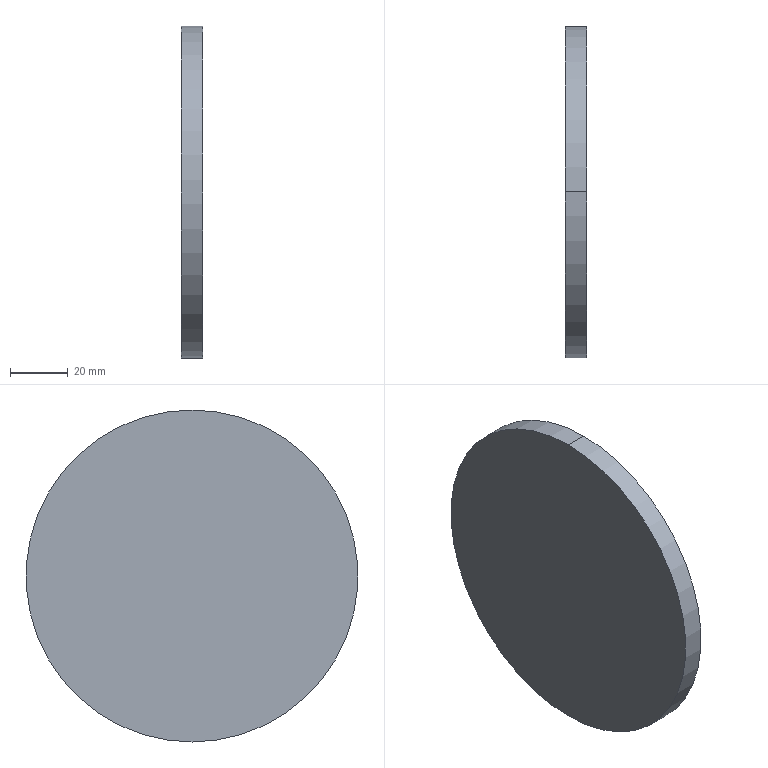Part | STEP file | G3L22N30-MM02TNNTNXH6-Part-9 | 1 solid | 4 faces | box 7.5 x 115 x 115 mm | volume 77902 mm3 | cylinder 2 | plane 2 | commonest cylinder face diameters 115 x2
STEP:
#1=CARTESIAN_POINT('',(-90.5,-19.,-57.5));
#2=VERTEX_POINT('',#1);
#3=CARTESIAN_POINT('',(-90.5,-19.,57.5));
#4=VERTEX_POINT('',#3);
#5=CARTESIAN_POINT('',(-90.5,-19.,0.));
#6=DIRECTION('',(1.,0.,0.));
#7=DIRECTION('',(0.,0.,-1.));
#8=AXIS2_PLACEMENT_3D('',#5,#6,#7);
#9=CIRCLE('',#8,57.5);
#10=EDGE_CURVE('',#2,#4,#9,.T.);
#11=ORIENTED_EDGE('',*,*,#10,.T.);
#12=CARTESIAN_POINT('',(-83.,-19.,57.5));
#13=VERTEX_POINT('',#12);
#14=CARTESIAN_POINT('',(-83.,-19.,57.5));
#15=DIRECTION('',(1.,0.,0.));
#16=VECTOR('',#15,1000.);
#17=LINE('',#14,#16);
#18=EDGE_CURVE('',#4,#13,#17,.T.);
#19=ORIENTED_EDGE('',*,*,#18,.T.);
#20=CARTESIAN_POINT('',(-83.,-19.,-57.5));
#21=VERTEX_POINT('',#20);
#22=CARTESIAN_POINT('',(-83.,-19.,0.));
#23=DIRECTION('',(1.,0.,0.));
#24=DIRECTION('',(0.,0.,-1.));
#25=AXIS2_PLACEMENT_3D('',#22,#23,#24);
#26=CIRCLE('',#25,57.5);
#27=EDGE_CURVE('',#21,#13,#26,.T.);
#28=ORIENTED_EDGE('',*,*,#27,.F.);
#29=CARTESIAN_POINT('',(-83.,-19.,-57.5));
#30=DIRECTION('',(1.,0.,0.));
#31=VECTOR('',#30,1000.);
#32=LINE('',#29,#31);
#33=EDGE_CURVE('',#2,#21,#32,.T.);
#34=ORIENTED_EDGE('',*,*,#33,.F.);
#35=EDGE_LOOP('',(#11,#19,#28,#34));
#36=FACE_OUTER_BOUND('',#35,.T.);
#37=CARTESIAN_POINT('',(-83.,-19.,0.));
#38=DIRECTION('',(1.,0.,0.));
#39=DIRECTION('',(0.,0.,-1.));
#40=AXIS2_PLACEMENT_3D('',#37,#38,#39);
#41=CYLINDRICAL_SURFACE('',#40,57.5);
#42=ADVANCED_FACE('',(#36),#41,.T.);
#43=ORIENTED_EDGE('',*,*,#10,.F.);
#44=CARTESIAN_POINT('',(-90.5,-19.,0.));
#45=DIRECTION('',(1.,0.,0.));
#46=DIRECTION('',(0.,0.,-1.));
#47=AXIS2_PLACEMENT_3D('',#44,#45,#46);
#48=CIRCLE('',#47,57.5);
#49=EDGE_CURVE('',#4,#2,#48,.T.);
#50=ORIENTED_EDGE('',*,*,#49,.F.);
#51=EDGE_LOOP('',(#43,#50));
#52=FACE_OUTER_BOUND('',#51,.T.);
#53=CARTESIAN_POINT('',(-90.5,-19.,0.));
#54=DIRECTION('',(1.,0.,0.));
#55=DIRECTION('',(0.,0.,-1.));
#56=AXIS2_PLACEMENT_3D('',#53,#54,#55);
#57=PLANE('',#56);
#58=ADVANCED_FACE('',(#52),#57,.F.);
#59=ORIENTED_EDGE('',*,*,#18,.F.);
#60=ORIENTED_EDGE('',*,*,#49,.T.);
#61=ORIENTED_EDGE('',*,*,#33,.T.);
#62=CARTESIAN_POINT('',(-83.,-19.,0.));
#63=DIRECTION('',(1.,0.,0.));
#64=DIRECTION('',(0.,0.,-1.));
#65=AXIS2_PLACEMENT_3D('',#62,#63,#64);
#66=CIRCLE('',#65,57.5);
#67=EDGE_CURVE('',#13,#21,#66,.T.);
#68=ORIENTED_EDGE('',*,*,#67,.F.);
#69=EDGE_LOOP('',(#59,#60,#61,#68));
#70=FACE_OUTER_BOUND('',#69,.T.);
#71=CARTESIAN_POINT('',(-83.,-19.,0.));
#72=DIRECTION('',(1.,0.,0.));
#73=DIRECTION('',(0.,0.,-1.));
#74=AXIS2_PLACEMENT_3D('',#71,#72,#73);
#75=CYLINDRICAL_SURFACE('',#74,57.5);
#76=ADVANCED_FACE('',(#70),#75,.T.);
#77=ORIENTED_EDGE('',*,*,#27,.T.);
#78=ORIENTED_EDGE('',*,*,#67,.T.);
#79=EDGE_LOOP('',(#77,#78));
#80=FACE_OUTER_BOUND('',#79,.T.);
#81=CARTESIAN_POINT('',(-83.,38.5,0.));
#82=DIRECTION('',(-1.,0.,0.));
#83=DIRECTION('',(0.,0.,1.));
#84=AXIS2_PLACEMENT_3D('',#81,#82,#83);
#85=PLANE('',#84);
#86=ADVANCED_FACE('',(#80),#85,.F.);
#87=CLOSED_SHELL('',(#42,#58,#76,#86));
#88=MANIFOLD_SOLID_BREP('',#87);
#89=CARTESIAN_POINT('',(0.,0.,0.));
#90=DIRECTION('',(0.,0.,1.));
#91=DIRECTION('',(1.,0.,0.));
#92=AXIS2_PLACEMENT_3D('',#89,#90,#91);
#93=(LENGTH_UNIT()NAMED_UNIT(*)SI_UNIT(.MILLI.,.METRE.));
#94=UNCERTAINTY_MEASURE_WITH_UNIT(LENGTH_MEASURE(0.00001),#93,'','');
#95=(NAMED_UNIT(*)PLANE_ANGLE_UNIT()SI_UNIT($,.RADIAN.));
#96=(NAMED_UNIT(*)SI_UNIT($,.STERADIAN.)SOLID_ANGLE_UNIT());
#97=(GEOMETRIC_REPRESENTATION_CONTEXT(3)GLOBAL_UNCERTAINTY_ASSIGNED_CONTEXT((#94))GLOBAL_UNIT_ASSIGNED_CONTEXT((#93,#95,#96))REPRESENTATION_CONTEXT('',''));
#98=ADVANCED_BREP_SHAPE_REPRESENTATION('',(#88,#92),#97);